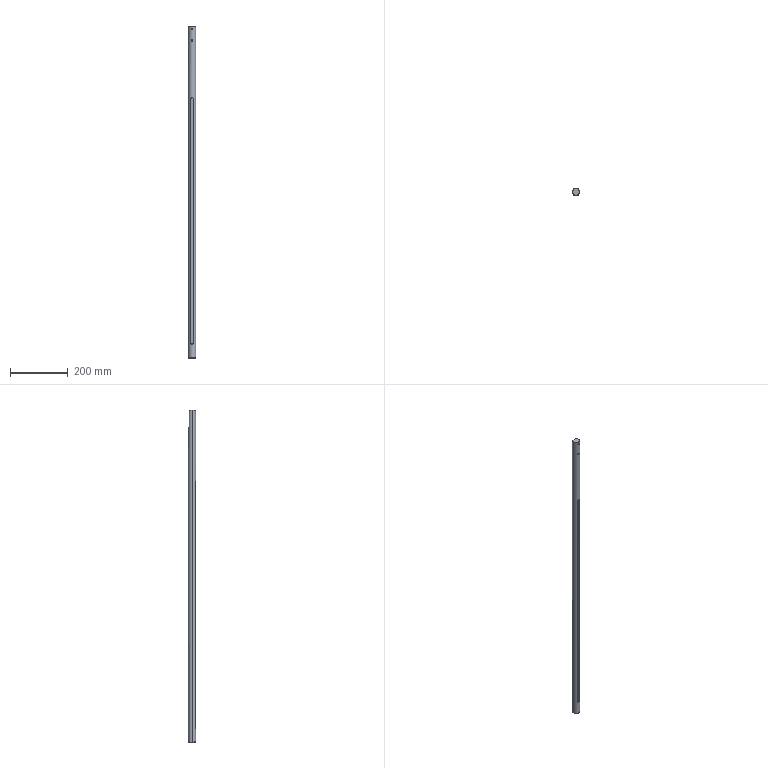Part | STEP file | Extension support shaft | 1 solid | 21 faces | box 25 x 25 x 1150 mm | volume 526631 mm3 | cylinder 9 | plane 7 | cone 5 | commonest cylinder face diameters 5 x4 7 x3 25 x2